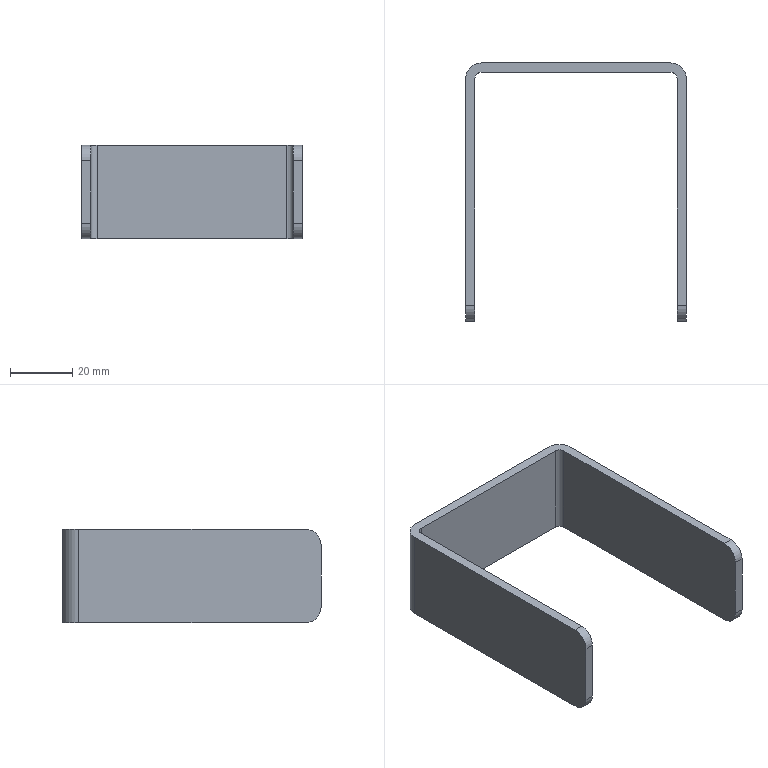Part | NX | features BLEND 1, DATUM_CSYS 1, EXTRACT_DATUM_PLANE 1, EXTRUDE 1, SHELL 1, SKETCH 1 | 1 solid | 18 faces | box 71 x 83 x 30 mm | volume 20455 mm3 | plane 10 | cylinder 8 | commonest cylinder face diameters 10 x6 4 x2
STEP:
#1=CARTESIAN_POINT('',(-32.5,-5.,-15.));
#2=VERTEX_POINT('',#1);
#3=CARTESIAN_POINT('',(-35.5,-5.,-15.));
#4=VERTEX_POINT('',#3);
#5=CARTESIAN_POINT('',(35.5,-5.,-15.));
#6=DIRECTION('',(-1.,0.,0.));
#7=VECTOR('',#6,1000.);
#8=LINE('',#5,#7);
#9=EDGE_CURVE('',#2,#4,#8,.T.);
#10=ORIENTED_EDGE('',*,*,#9,.F.);
#11=CARTESIAN_POINT('',(-32.5,-10.,-10.));
#12=VERTEX_POINT('',#11);
#13=CARTESIAN_POINT('',(-32.5,-5.,-10.));
#14=DIRECTION('',(-1.,0.,0.));
#15=DIRECTION('',(0.,0.,1.));
#16=AXIS2_PLACEMENT_3D('',#13,#14,#15);
#17=CIRCLE('',#16,5.);
#18=EDGE_CURVE('',#2,#12,#17,.T.);
#19=ORIENTED_EDGE('',*,*,#18,.T.);
#20=CARTESIAN_POINT('',(-35.5,-10.,-10.));
#21=VERTEX_POINT('',#20);
#22=CARTESIAN_POINT('',(35.5,-10.,-10.));
#23=DIRECTION('',(-1.,0.,0.));
#24=VECTOR('',#23,1000.);
#25=LINE('',#22,#24);
#26=EDGE_CURVE('',#12,#21,#25,.T.);
#27=ORIENTED_EDGE('',*,*,#26,.T.);
#28=CARTESIAN_POINT('',(-35.5,-5.,-10.));
#29=DIRECTION('',(-1.,0.,0.));
#30=DIRECTION('',(0.,0.,-1.));
#31=AXIS2_PLACEMENT_3D('',#28,#29,#30);
#32=CIRCLE('',#31,5.);
#33=EDGE_CURVE('',#4,#21,#32,.T.);
#34=ORIENTED_EDGE('',*,*,#33,.F.);
#35=EDGE_LOOP('',(#10,#19,#27,#34));
#36=FACE_BOUND('',#35,.T.);
#37=CARTESIAN_POINT('',(35.5,-5.,-10.));
#38=DIRECTION('',(-1.,0.,0.));
#39=DIRECTION('',(0.,0.,1.));
#40=AXIS2_PLACEMENT_3D('',#37,#38,#39);
#41=CYLINDRICAL_SURFACE('',#40,5.);
#42=ADVANCED_FACE('',(#36),#41,.T.);
#43=ORIENTED_EDGE('',*,*,#26,.F.);
#44=CARTESIAN_POINT('',(-32.5,-10.,10.));
#45=VERTEX_POINT('',#44);
#46=CARTESIAN_POINT('',(-32.5,-10.,-10.));
#47=DIRECTION('',(0.,0.,1.));
#48=VECTOR('',#47,1000.);
#49=LINE('',#46,#48);
#50=EDGE_CURVE('',#12,#45,#49,.T.);
#51=ORIENTED_EDGE('',*,*,#50,.T.);
#52=CARTESIAN_POINT('',(-35.5,-10.,10.));
#53=VERTEX_POINT('',#52);
#54=CARTESIAN_POINT('',(35.5,-10.,10.));
#55=DIRECTION('',(-1.,0.,0.));
#56=VECTOR('',#55,1000.);
#57=LINE('',#54,#56);
#58=EDGE_CURVE('',#45,#53,#57,.T.);
#59=ORIENTED_EDGE('',*,*,#58,.T.);
#60=CARTESIAN_POINT('',(-35.5,-10.,-10.));
#61=DIRECTION('',(0.,0.,1.));
#62=VECTOR('',#61,1000.);
#63=LINE('',#60,#62);
#64=EDGE_CURVE('',#21,#53,#63,.T.);
#65=ORIENTED_EDGE('',*,*,#64,.F.);
#66=EDGE_LOOP('',(#43,#51,#59,#65));
#67=FACE_BOUND('',#66,.T.);
#68=CARTESIAN_POINT('',(35.5,-10.,-10.));
#69=DIRECTION('',(0.,-1.,0.));
#70=DIRECTION('',(0.,0.,-1.));
#71=AXIS2_PLACEMENT_3D('',#68,#69,#70);
#72=PLANE('',#71);
#73=ADVANCED_FACE('',(#67),#72,.T.);
#74=ORIENTED_EDGE('',*,*,#58,.F.);
#75=CARTESIAN_POINT('',(-32.5,-5.,15.));
#76=VERTEX_POINT('',#75);
#77=CARTESIAN_POINT('',(-32.5,-5.,10.));
#78=DIRECTION('',(-1.,0.,0.));
#79=DIRECTION('',(0.,0.,1.));
#80=AXIS2_PLACEMENT_3D('',#77,#78,#79);
#81=CIRCLE('',#80,5.);
#82=EDGE_CURVE('',#45,#76,#81,.T.);
#83=ORIENTED_EDGE('',*,*,#82,.T.);
#84=CARTESIAN_POINT('',(-35.5,-5.,15.));
#85=VERTEX_POINT('',#84);
#86=CARTESIAN_POINT('',(35.5,-5.,15.));
#87=DIRECTION('',(-1.,0.,0.));
#88=VECTOR('',#87,1000.);
#89=LINE('',#86,#88);
#90=EDGE_CURVE('',#76,#85,#89,.T.);
#91=ORIENTED_EDGE('',*,*,#90,.T.);
#92=CARTESIAN_POINT('',(-35.5,-5.,10.));
#93=DIRECTION('',(-1.,0.,0.));
#94=DIRECTION('',(0.,-1.,0.));
#95=AXIS2_PLACEMENT_3D('',#92,#93,#94);
#96=CIRCLE('',#95,5.);
#97=EDGE_CURVE('',#53,#85,#96,.T.);
#98=ORIENTED_EDGE('',*,*,#97,.F.);
#99=EDGE_LOOP('',(#74,#83,#91,#98));
#100=FACE_BOUND('',#99,.T.);
#101=CARTESIAN_POINT('',(35.5,-5.,10.));
#102=DIRECTION('',(-1.,0.,0.));
#103=DIRECTION('',(0.,0.,1.));
#104=AXIS2_PLACEMENT_3D('',#101,#102,#103);
#105=CYLINDRICAL_SURFACE('',#104,5.);
#106=ADVANCED_FACE('',(#100),#105,.T.);
#107=CARTESIAN_POINT('',(32.5,-5.,15.));
#108=VERTEX_POINT('',#107);
#109=CARTESIAN_POINT('',(32.5,68.,15.));
#110=VERTEX_POINT('',#109);
#111=CARTESIAN_POINT('',(32.5,-5.,15.));
#112=DIRECTION('',(0.,1.,0.));
#113=VECTOR('',#112,1000.);
#114=LINE('',#111,#113);
#115=EDGE_CURVE('',#108,#110,#114,.T.);
#116=ORIENTED_EDGE('',*,*,#115,.F.);
#117=CARTESIAN_POINT('',(35.5,-5.,15.));
#118=VERTEX_POINT('',#117);
#119=CARTESIAN_POINT('',(35.5,-5.,15.));
#120=DIRECTION('',(-1.,0.,0.));
#121=VECTOR('',#120,1000.);
#122=LINE('',#119,#121);
#123=EDGE_CURVE('',#118,#108,#122,.T.);
#124=ORIENTED_EDGE('',*,*,#123,.F.);
#125=CARTESIAN_POINT('',(35.5,68.,15.));
#126=VERTEX_POINT('',#125);
#127=CARTESIAN_POINT('',(35.5,-5.,15.));
#128=DIRECTION('',(0.,1.,0.));
#129=VECTOR('',#128,1000.);
#130=LINE('',#127,#129);
#131=EDGE_CURVE('',#118,#126,#130,.T.);
#132=ORIENTED_EDGE('',*,*,#131,.T.);
#133=CARTESIAN_POINT('',(30.5,73.,15.));
#134=VERTEX_POINT('',#133);
#135=CARTESIAN_POINT('',(30.5,68.,15.));
#136=DIRECTION('',(0.,0.,1.));
#137=DIRECTION('',(1.,0.,0.));
#138=AXIS2_PLACEMENT_3D('',#135,#136,#137);
#139=CIRCLE('',#138,5.);
#140=EDGE_CURVE('',#126,#134,#139,.T.);
#141=ORIENTED_EDGE('',*,*,#140,.T.);
#142=CARTESIAN_POINT('',(-30.5,73.,15.));
#143=VERTEX_POINT('',#142);
#144=CARTESIAN_POINT('',(35.5,73.,15.));
#145=DIRECTION('',(-1.,0.,0.));
#146=VECTOR('',#145,1000.);
#147=LINE('',#144,#146);
#148=EDGE_CURVE('',#134,#143,#147,.T.);
#149=ORIENTED_EDGE('',*,*,#148,.T.);
#150=CARTESIAN_POINT('',(-35.5,68.,15.));
#151=VERTEX_POINT('',#150);
#152=CARTESIAN_POINT('',(-30.5,68.,15.));
#153=DIRECTION('',(0.,0.,1.));
#154=DIRECTION('',(1.,0.,0.));
#155=AXIS2_PLACEMENT_3D('',#152,#153,#154);
#156=CIRCLE('',#155,5.);
#157=EDGE_CURVE('',#143,#151,#156,.T.);
#158=ORIENTED_EDGE('',*,*,#157,.T.);
#159=CARTESIAN_POINT('',(-35.5,68.,15.));
#160=DIRECTION('',(0.,1.,0.));
#161=VECTOR('',#160,1000.);
#162=LINE('',#159,#161);
#163=EDGE_CURVE('',#85,#151,#162,.T.);
#164=ORIENTED_EDGE('',*,*,#163,.F.);
#165=ORIENTED_EDGE('',*,*,#90,.F.);
#166=CARTESIAN_POINT('',(-32.5,68.,15.));
#167=VERTEX_POINT('',#166);
#168=CARTESIAN_POINT('',(-32.5,-5.,15.));
#169=DIRECTION('',(0.,1.,0.));
#170=VECTOR('',#169,1000.);
#171=LINE('',#168,#170);
#172=EDGE_CURVE('',#76,#167,#171,.T.);
#173=ORIENTED_EDGE('',*,*,#172,.T.);
#174=CARTESIAN_POINT('',(-30.5,70.,15.));
#175=VERTEX_POINT('',#174);
#176=CARTESIAN_POINT('',(-30.5,68.,15.));
#177=DIRECTION('',(0.,0.,1.));
#178=DIRECTION('',(1.,0.,0.));
#179=AXIS2_PLACEMENT_3D('',#176,#177,#178);
#180=CIRCLE('',#179,2.);
#181=EDGE_CURVE('',#175,#167,#180,.T.);
#182=ORIENTED_EDGE('',*,*,#181,.F.);
#183=CARTESIAN_POINT('',(30.5,70.,15.));
#184=VERTEX_POINT('',#183);
#185=CARTESIAN_POINT('',(35.5,70.,15.));
#186=DIRECTION('',(-1.,0.,0.));
#187=VECTOR('',#186,1000.);
#188=LINE('',#185,#187);
#189=EDGE_CURVE('',#184,#175,#188,.T.);
#190=ORIENTED_EDGE('',*,*,#189,.F.);
#191=CARTESIAN_POINT('',(30.5,68.,15.));
#192=DIRECTION('',(0.,0.,1.));
#193=DIRECTION('',(1.,0.,0.));
#194=AXIS2_PLACEMENT_3D('',#191,#192,#193);
#195=CIRCLE('',#194,2.);
#196=EDGE_CURVE('',#110,#184,#195,.T.);
#197=ORIENTED_EDGE('',*,*,#196,.F.);
#198=EDGE_LOOP('',(#116,#124,#132,#141,#149,#158,#164,#165,#173,#182,#190,#197));
#199=FACE_BOUND('',#198,.T.);
#200=CARTESIAN_POINT('',(35.5,68.,15.));
#201=DIRECTION('',(0.,0.,1.));
#202=DIRECTION('',(1.,0.,0.));
#203=AXIS2_PLACEMENT_3D('',#200,#201,#202);
#204=PLANE('',#203);
#205=ADVANCED_FACE('',(#199),#204,.T.);
#206=ORIENTED_EDGE('',*,*,#148,.F.);
#207=CARTESIAN_POINT('',(30.5,73.,-15.));
#208=VERTEX_POINT('',#207);
#209=CARTESIAN_POINT('',(30.5,73.,-15.));
#210=DIRECTION('',(0.,0.,-1.));
#211=VECTOR('',#210,1000.);
#212=LINE('',#209,#211);
#213=EDGE_CURVE('',#134,#208,#212,.T.);
#214=ORIENTED_EDGE('',*,*,#213,.T.);
#215=CARTESIAN_POINT('',(-30.5,73.,-15.));
#216=VERTEX_POINT('',#215);
#217=CARTESIAN_POINT('',(35.5,73.,-15.));
#218=DIRECTION('',(-1.,0.,0.));
#219=VECTOR('',#218,1000.);
#220=LINE('',#217,#219);
#221=EDGE_CURVE('',#208,#216,#220,.T.);
#222=ORIENTED_EDGE('',*,*,#221,.T.);
#223=CARTESIAN_POINT('',(-30.5,73.,15.));
#224=DIRECTION('',(0.,0.,-1.));
#225=VECTOR('',#224,1000.);
#226=LINE('',#223,#225);
#227=EDGE_CURVE('',#216,#143,#226,.F.);
#228=ORIENTED_EDGE('',*,*,#227,.T.);
#229=EDGE_LOOP('',(#206,#214,#222,#228));
#230=FACE_BOUND('',#229,.T.);
#231=CARTESIAN_POINT('',(35.5,73.,15.));
#232=DIRECTION('',(0.,1.,0.));
#233=DIRECTION('',(0.,0.,1.));
#234=AXIS2_PLACEMENT_3D('',#231,#232,#233);
#235=PLANE('',#234);
#236=ADVANCED_FACE('',(#230),#235,.T.);
#237=CARTESIAN_POINT('',(32.5,68.,-15.));
#238=VERTEX_POINT('',#237);
#239=CARTESIAN_POINT('',(32.5,-5.,-15.));
#240=VERTEX_POINT('',#239);
#241=CARTESIAN_POINT('',(32.5,-5.,-15.));
#242=DIRECTION('',(0.,-1.,0.));
#243=VECTOR('',#242,1000.);
#244=LINE('',#241,#243);
#245=EDGE_CURVE('',#238,#240,#244,.T.);
#246=ORIENTED_EDGE('',*,*,#245,.F.);
#247=CARTESIAN_POINT('',(30.5,70.,-15.));
#248=VERTEX_POINT('',#247);
#249=CARTESIAN_POINT('',(30.5,68.,-15.));
#250=DIRECTION('',(0.,0.,-1.));
#251=DIRECTION('',(-1.,0.,0.));
#252=AXIS2_PLACEMENT_3D('',#249,#250,#251);
#253=CIRCLE('',#252,2.);
#254=EDGE_CURVE('',#248,#238,#253,.T.);
#255=ORIENTED_EDGE('',*,*,#254,.F.);
#256=CARTESIAN_POINT('',(-30.5,70.,-15.));
#257=VERTEX_POINT('',#256);
#258=CARTESIAN_POINT('',(35.5,70.,-15.));
#259=DIRECTION('',(-1.,0.,0.));
#260=VECTOR('',#259,1000.);
#261=LINE('',#258,#260);
#262=EDGE_CURVE('',#248,#257,#261,.T.);
#263=ORIENTED_EDGE('',*,*,#262,.T.);
#264=CARTESIAN_POINT('',(-32.5,68.,-15.));
#265=VERTEX_POINT('',#264);
#266=CARTESIAN_POINT('',(-30.5,68.,-15.));
#267=DIRECTION('',(0.,0.,-1.));
#268=DIRECTION('',(-1.,0.,0.));
#269=AXIS2_PLACEMENT_3D('',#266,#267,#268);
#270=CIRCLE('',#269,2.);
#271=EDGE_CURVE('',#265,#257,#270,.T.);
#272=ORIENTED_EDGE('',*,*,#271,.F.);
#273=CARTESIAN_POINT('',(-32.5,-5.,-15.));
#274=DIRECTION('',(0.,-1.,0.));
#275=VECTOR('',#274,1000.);
#276=LINE('',#273,#275);
#277=EDGE_CURVE('',#265,#2,#276,.T.);
#278=ORIENTED_EDGE('',*,*,#277,.T.);
#279=ORIENTED_EDGE('',*,*,#9,.T.);
#280=CARTESIAN_POINT('',(-35.5,68.,-15.));
#281=VERTEX_POINT('',#280);
#282=CARTESIAN_POINT('',(-35.5,68.,-15.));
#283=DIRECTION('',(0.,-1.,0.));
#284=VECTOR('',#283,1000.);
#285=LINE('',#282,#284);
#286=EDGE_CURVE('',#281,#4,#285,.T.);
#287=ORIENTED_EDGE('',*,*,#286,.F.);
#288=CARTESIAN_POINT('',(-30.5,68.,-15.));
#289=DIRECTION('',(0.,0.,-1.));
#290=DIRECTION('',(-1.,0.,0.));
#291=AXIS2_PLACEMENT_3D('',#288,#289,#290);
#292=CIRCLE('',#291,5.);
#293=EDGE_CURVE('',#281,#216,#292,.T.);
#294=ORIENTED_EDGE('',*,*,#293,.T.);
#295=ORIENTED_EDGE('',*,*,#221,.F.);
#296=CARTESIAN_POINT('',(35.5,68.,-15.));
#297=VERTEX_POINT('',#296);
#298=CARTESIAN_POINT('',(30.5,68.,-15.));
#299=DIRECTION('',(0.,0.,-1.));
#300=DIRECTION('',(-1.,0.,0.));
#301=AXIS2_PLACEMENT_3D('',#298,#299,#300);
#302=CIRCLE('',#301,5.);
#303=EDGE_CURVE('',#208,#297,#302,.T.);
#304=ORIENTED_EDGE('',*,*,#303,.T.);
#305=CARTESIAN_POINT('',(35.5,-5.,-15.));
#306=VERTEX_POINT('',#305);
#307=CARTESIAN_POINT('',(35.5,73.,-15.));
#308=DIRECTION('',(0.,-1.,0.));
#309=VECTOR('',#308,1000.);
#310=LINE('',#307,#309);
#311=EDGE_CURVE('',#297,#306,#310,.T.);
#312=ORIENTED_EDGE('',*,*,#311,.T.);
#313=CARTESIAN_POINT('',(35.5,-5.,-15.));
#314=DIRECTION('',(-1.,0.,0.));
#315=VECTOR('',#314,1000.);
#316=LINE('',#313,#315);
#317=EDGE_CURVE('',#306,#240,#316,.T.);
#318=ORIENTED_EDGE('',*,*,#317,.T.);
#319=EDGE_LOOP('',(#246,#255,#263,#272,#278,#279,#287,#294,#295,#304,#312,#318));
#320=FACE_BOUND('',#319,.T.);
#321=CARTESIAN_POINT('',(35.5,68.,-15.));
#322=DIRECTION('',(0.,0.,-1.));
#323=DIRECTION('',(-1.,0.,0.));
#324=AXIS2_PLACEMENT_3D('',#321,#322,#323);
#325=PLANE('',#324);
#326=ADVANCED_FACE('',(#320),#325,.T.);
#327=CARTESIAN_POINT('',(32.5,-10.,-10.));
#328=VERTEX_POINT('',#327);
#329=CARTESIAN_POINT('',(32.5,-5.,-10.));
#330=DIRECTION('',(-1.,0.,0.));
#331=DIRECTION('',(0.,0.,1.));
#332=AXIS2_PLACEMENT_3D('',#329,#330,#331);
#333=CIRCLE('',#332,5.);
#334=EDGE_CURVE('',#240,#328,#333,.T.);
#335=ORIENTED_EDGE('',*,*,#334,.F.);
#336=ORIENTED_EDGE('',*,*,#317,.F.);
#337=CARTESIAN_POINT('',(35.5,-10.,-10.));
#338=VERTEX_POINT('',#337);
#339=CARTESIAN_POINT('',(35.5,-5.,-10.));
#340=DIRECTION('',(-1.,0.,0.));
#341=DIRECTION('',(0.,0.,-1.));
#342=AXIS2_PLACEMENT_3D('',#339,#340,#341);
#343=CIRCLE('',#342,5.);
#344=EDGE_CURVE('',#306,#338,#343,.T.);
#345=ORIENTED_EDGE('',*,*,#344,.T.);
#346=CARTESIAN_POINT('',(35.5,-10.,-10.));
#347=DIRECTION('',(-1.,0.,0.));
#348=VECTOR('',#347,1000.);
#349=LINE('',#346,#348);
#350=EDGE_CURVE('',#338,#328,#349,.T.);
#351=ORIENTED_EDGE('',*,*,#350,.T.);
#352=EDGE_LOOP('',(#335,#336,#345,#351));
#353=FACE_BOUND('',#352,.T.);
#354=CARTESIAN_POINT('',(35.5,-5.,-10.));
#355=DIRECTION('',(-1.,0.,0.));
#356=DIRECTION('',(0.,0.,1.));
#357=AXIS2_PLACEMENT_3D('',#354,#355,#356);
#358=CYLINDRICAL_SURFACE('',#357,5.);
#359=ADVANCED_FACE('',(#353),#358,.T.);
#360=CARTESIAN_POINT('',(32.5,-10.,10.));
#361=VERTEX_POINT('',#360);
#362=CARTESIAN_POINT('',(32.5,-10.,-10.));
#363=DIRECTION('',(0.,0.,1.));
#364=VECTOR('',#363,1000.);
#365=LINE('',#362,#364);
#366=EDGE_CURVE('',#328,#361,#365,.T.);
#367=ORIENTED_EDGE('',*,*,#366,.F.);
#368=ORIENTED_EDGE('',*,*,#350,.F.);
#369=CARTESIAN_POINT('',(35.5,-10.,10.));
#370=VERTEX_POINT('',#369);
#371=CARTESIAN_POINT('',(35.5,-10.,-10.));
#372=DIRECTION('',(0.,0.,1.));
#373=VECTOR('',#372,1000.);
#374=LINE('',#371,#373);
#375=EDGE_CURVE('',#338,#370,#374,.T.);
#376=ORIENTED_EDGE('',*,*,#375,.T.);
#377=CARTESIAN_POINT('',(35.5,-10.,10.));
#378=DIRECTION('',(-1.,0.,0.));
#379=VECTOR('',#378,1000.);
#380=LINE('',#377,#379);
#381=EDGE_CURVE('',#370,#361,#380,.T.);
#382=ORIENTED_EDGE('',*,*,#381,.T.);
#383=EDGE_LOOP('',(#367,#368,#376,#382));
#384=FACE_BOUND('',#383,.T.);
#385=CARTESIAN_POINT('',(35.5,-10.,-10.));
#386=DIRECTION('',(0.,-1.,0.));
#387=DIRECTION('',(0.,0.,-1.));
#388=AXIS2_PLACEMENT_3D('',#385,#386,#387);
#389=PLANE('',#388);
#390=ADVANCED_FACE('',(#384),#389,.T.);
#391=CARTESIAN_POINT('',(32.5,-5.,10.));
#392=DIRECTION('',(-1.,0.,0.));
#393=DIRECTION('',(0.,0.,1.));
#394=AXIS2_PLACEMENT_3D('',#391,#392,#393);
#395=CIRCLE('',#394,5.);
#396=EDGE_CURVE('',#361,#108,#395,.T.);
#397=ORIENTED_EDGE('',*,*,#396,.F.);
#398=ORIENTED_EDGE('',*,*,#381,.F.);
#399=CARTESIAN_POINT('',(35.5,-5.,10.));
#400=DIRECTION('',(-1.,0.,0.));
#401=DIRECTION('',(0.,-1.,0.));
#402=AXIS2_PLACEMENT_3D('',#399,#400,#401);
#403=CIRCLE('',#402,5.);
#404=EDGE_CURVE('',#370,#118,#403,.T.);
#405=ORIENTED_EDGE('',*,*,#404,.T.);
#406=ORIENTED_EDGE('',*,*,#123,.T.);
#407=EDGE_LOOP('',(#397,#398,#405,#406));
#408=FACE_BOUND('',#407,.T.);
#409=CARTESIAN_POINT('',(35.5,-5.,10.));
#410=DIRECTION('',(-1.,0.,0.));
#411=DIRECTION('',(0.,0.,1.));
#412=AXIS2_PLACEMENT_3D('',#409,#410,#411);
#413=CYLINDRICAL_SURFACE('',#412,5.);
#414=ADVANCED_FACE('',(#408),#413,.T.);
#415=ORIENTED_EDGE('',*,*,#311,.F.);
#416=CARTESIAN_POINT('',(35.5,68.,15.));
#417=DIRECTION('',(0.,0.,-1.));
#418=VECTOR('',#417,1000.);
#419=LINE('',#416,#418);
#420=EDGE_CURVE('',#297,#126,#419,.F.);
#421=ORIENTED_EDGE('',*,*,#420,.T.);
#422=ORIENTED_EDGE('',*,*,#131,.F.);
#423=ORIENTED_EDGE('',*,*,#404,.F.);
#424=ORIENTED_EDGE('',*,*,#375,.F.);
#425=ORIENTED_EDGE('',*,*,#344,.F.);
#426=EDGE_LOOP('',(#415,#421,#422,#423,#424,#425));
#427=FACE_BOUND('',#426,.T.);
#428=CARTESIAN_POINT('',(35.5,-5.,-10.));
#429=DIRECTION('',(-1.,0.,0.));
#430=DIRECTION('',(0.,0.,1.));
#431=AXIS2_PLACEMENT_3D('',#428,#429,#430);
#432=PLANE('',#431);
#433=ADVANCED_FACE('',(#427),#432,.F.);
#434=ORIENTED_EDGE('',*,*,#163,.T.);
#435=CARTESIAN_POINT('',(-35.5,68.,-10.));
#436=DIRECTION('',(0.,0.,-1.));
#437=VECTOR('',#436,1000.);
#438=LINE('',#435,#437);
#439=EDGE_CURVE('',#151,#281,#438,.T.);
#440=ORIENTED_EDGE('',*,*,#439,.T.);
#441=ORIENTED_EDGE('',*,*,#286,.T.);
#442=ORIENTED_EDGE('',*,*,#33,.T.);
#443=ORIENTED_EDGE('',*,*,#64,.T.);
#444=ORIENTED_EDGE('',*,*,#97,.T.);
#445=EDGE_LOOP('',(#434,#440,#441,#442,#443,#444));
#446=FACE_BOUND('',#445,.T.);
#447=CARTESIAN_POINT('',(-35.5,-5.,-10.));
#448=DIRECTION('',(-1.,0.,0.));
#449=DIRECTION('',(0.,0.,1.));
#450=AXIS2_PLACEMENT_3D('',#447,#448,#449);
#451=PLANE('',#450);
#452=ADVANCED_FACE('',(#446),#451,.T.);
#453=ORIENTED_EDGE('',*,*,#140,.F.);
#454=ORIENTED_EDGE('',*,*,#420,.F.);
#455=ORIENTED_EDGE('',*,*,#303,.F.);
#456=ORIENTED_EDGE('',*,*,#213,.F.);
#457=EDGE_LOOP('',(#453,#454,#455,#456));
#458=FACE_BOUND('',#457,.T.);
#459=CARTESIAN_POINT('',(30.5,68.,15.));
#460=DIRECTION('',(0.,0.,1.));
#461=DIRECTION('',(1.,0.,0.));
#462=AXIS2_PLACEMENT_3D('',#459,#460,#461);
#463=CYLINDRICAL_SURFACE('',#462,5.);
#464=ADVANCED_FACE('',(#458),#463,.T.);
#465=ORIENTED_EDGE('',*,*,#157,.F.);
#466=ORIENTED_EDGE('',*,*,#227,.F.);
#467=ORIENTED_EDGE('',*,*,#293,.F.);
#468=ORIENTED_EDGE('',*,*,#439,.F.);
#469=EDGE_LOOP('',(#465,#466,#467,#468));
#470=FACE_BOUND('',#469,.T.);
#471=CARTESIAN_POINT('',(-30.5,68.,-10.));
#472=DIRECTION('',(0.,0.,-1.));
#473=DIRECTION('',(-1.,0.,0.));
#474=AXIS2_PLACEMENT_3D('',#471,#472,#473);
#475=CYLINDRICAL_SURFACE('',#474,5.);
#476=ADVANCED_FACE('',(#470),#475,.T.);
#477=ORIENTED_EDGE('',*,*,#189,.T.);
#478=CARTESIAN_POINT('',(-30.5,70.,15.));
#479=DIRECTION('',(0.,0.,1.));
#480=VECTOR('',#479,1000.);
#481=LINE('',#478,#480);
#482=EDGE_CURVE('',#257,#175,#481,.T.);
#483=ORIENTED_EDGE('',*,*,#482,.F.);
#484=ORIENTED_EDGE('',*,*,#262,.F.);
#485=CARTESIAN_POINT('',(30.5,70.,15.));
#486=DIRECTION('',(0.,0.,1.));
#487=VECTOR('',#486,1000.);
#488=LINE('',#485,#487);
#489=EDGE_CURVE('',#184,#248,#488,.F.);
#490=ORIENTED_EDGE('',*,*,#489,.F.);
#491=EDGE_LOOP('',(#477,#483,#484,#490));
#492=FACE_BOUND('',#491,.T.);
#493=CARTESIAN_POINT('',(35.5,70.,15.));
#494=DIRECTION('',(0.,1.,0.));
#495=DIRECTION('',(0.,0.,1.));
#496=AXIS2_PLACEMENT_3D('',#493,#494,#495);
#497=PLANE('',#496);
#498=ADVANCED_FACE('',(#492),#497,.F.);
#499=ORIENTED_EDGE('',*,*,#245,.T.);
#500=ORIENTED_EDGE('',*,*,#334,.T.);
#501=ORIENTED_EDGE('',*,*,#366,.T.);
#502=ORIENTED_EDGE('',*,*,#396,.T.);
#503=ORIENTED_EDGE('',*,*,#115,.T.);
#504=CARTESIAN_POINT('',(32.5,68.,-10.));
#505=DIRECTION('',(0.,0.,1.));
#506=VECTOR('',#505,1000.);
#507=LINE('',#504,#506);
#508=EDGE_CURVE('',#238,#110,#507,.T.);
#509=ORIENTED_EDGE('',*,*,#508,.F.);
#510=EDGE_LOOP('',(#499,#500,#501,#502,#503,#509));
#511=FACE_BOUND('',#510,.T.);
#512=CARTESIAN_POINT('',(32.5,-5.,-10.));
#513=DIRECTION('',(-1.,0.,0.));
#514=DIRECTION('',(0.,0.,1.));
#515=AXIS2_PLACEMENT_3D('',#512,#513,#514);
#516=PLANE('',#515);
#517=ADVANCED_FACE('',(#511),#516,.T.);
#518=ORIENTED_EDGE('',*,*,#172,.F.);
#519=ORIENTED_EDGE('',*,*,#82,.F.);
#520=ORIENTED_EDGE('',*,*,#50,.F.);
#521=ORIENTED_EDGE('',*,*,#18,.F.);
#522=ORIENTED_EDGE('',*,*,#277,.F.);
#523=CARTESIAN_POINT('',(-32.5,68.,-10.));
#524=DIRECTION('',(0.,0.,1.));
#525=VECTOR('',#524,1000.);
#526=LINE('',#523,#525);
#527=EDGE_CURVE('',#167,#265,#526,.F.);
#528=ORIENTED_EDGE('',*,*,#527,.F.);
#529=EDGE_LOOP('',(#518,#519,#520,#521,#522,#528));
#530=FACE_BOUND('',#529,.T.);
#531=CARTESIAN_POINT('',(-32.5,-5.,-10.));
#532=DIRECTION('',(-1.,0.,0.));
#533=DIRECTION('',(0.,0.,1.));
#534=AXIS2_PLACEMENT_3D('',#531,#532,#533);
#535=PLANE('',#534);
#536=ADVANCED_FACE('',(#530),#535,.F.);
#537=ORIENTED_EDGE('',*,*,#196,.T.);
#538=ORIENTED_EDGE('',*,*,#489,.T.);
#539=ORIENTED_EDGE('',*,*,#254,.T.);
#540=ORIENTED_EDGE('',*,*,#508,.T.);
#541=EDGE_LOOP('',(#537,#538,#539,#540));
#542=FACE_BOUND('',#541,.T.);
#543=CARTESIAN_POINT('',(30.5,68.,15.));
#544=DIRECTION('',(0.,0.,1.));
#545=DIRECTION('',(1.,0.,0.));
#546=AXIS2_PLACEMENT_3D('',#543,#544,#545);
#547=CYLINDRICAL_SURFACE('',#546,2.);
#548=ADVANCED_FACE('',(#542),#547,.F.);
#549=ORIENTED_EDGE('',*,*,#181,.T.);
#550=ORIENTED_EDGE('',*,*,#527,.T.);
#551=ORIENTED_EDGE('',*,*,#271,.T.);
#552=ORIENTED_EDGE('',*,*,#482,.T.);
#553=EDGE_LOOP('',(#549,#550,#551,#552));
#554=FACE_BOUND('',#553,.T.);
#555=CARTESIAN_POINT('',(-30.5,68.,-10.));
#556=DIRECTION('',(0.,0.,-1.));
#557=DIRECTION('',(-1.,0.,0.));
#558=AXIS2_PLACEMENT_3D('',#555,#556,#557);
#559=CYLINDRICAL_SURFACE('',#558,2.);
#560=ADVANCED_FACE('',(#554),#559,.F.);
#561=CLOSED_SHELL('',(#42,#73,#106,#205,#236,#326,#359,#390,#414,#433,#452,#464,#476,#498,#517,#536,#548,#560));
#562=MANIFOLD_SOLID_BREP('',#561);
#563=(LENGTH_UNIT()NAMED_UNIT(*)SI_UNIT(.MILLI.,.METRE.));
#564=UNCERTAINTY_MEASURE_WITH_UNIT(LENGTH_MEASURE(0.00001),#563,'','');
#565=(NAMED_UNIT(*)PLANE_ANGLE_UNIT()SI_UNIT($,.RADIAN.));
#566=(NAMED_UNIT(*)SI_UNIT($,.STERADIAN.)SOLID_ANGLE_UNIT());
#567=(GEOMETRIC_REPRESENTATION_CONTEXT(3)GLOBAL_UNCERTAINTY_ASSIGNED_CONTEXT((#564))GLOBAL_UNIT_ASSIGNED_CONTEXT((#563,#565,#566))REPRESENTATION_CONTEXT('',''));
#568=ADVANCED_BREP_SHAPE_REPRESENTATION('',(#562),#567);